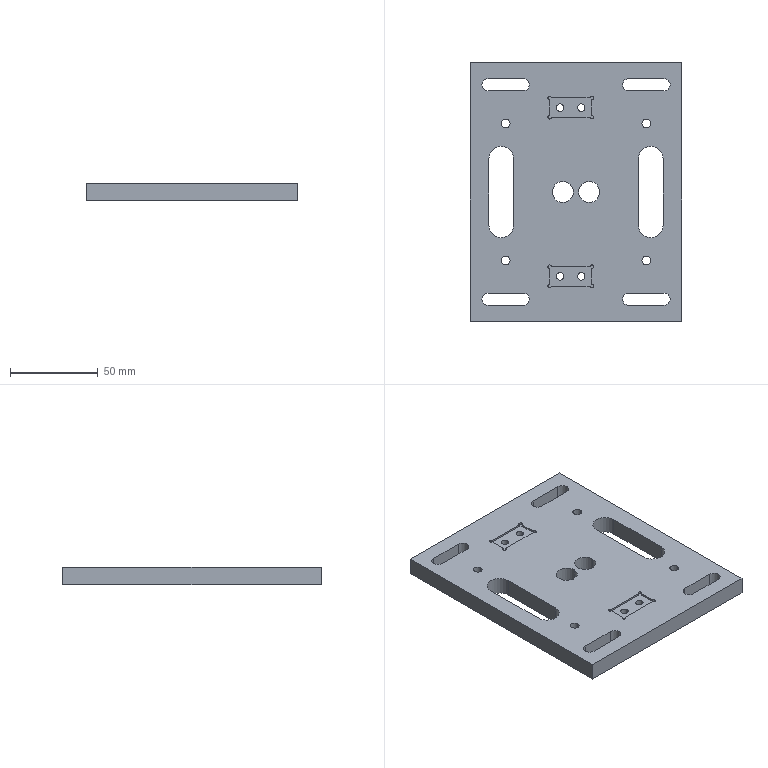Part | STEP file | GLSJ-10-48_default | 1 solid | 76 faces | box 120 x 147 x 10 mm | volume 151449 mm3 | cylinder 48 | plane 28 | commonest cylinder face diameters 2 x12 7 x12 4.2 x8 5 x8 12 x4 14 x4